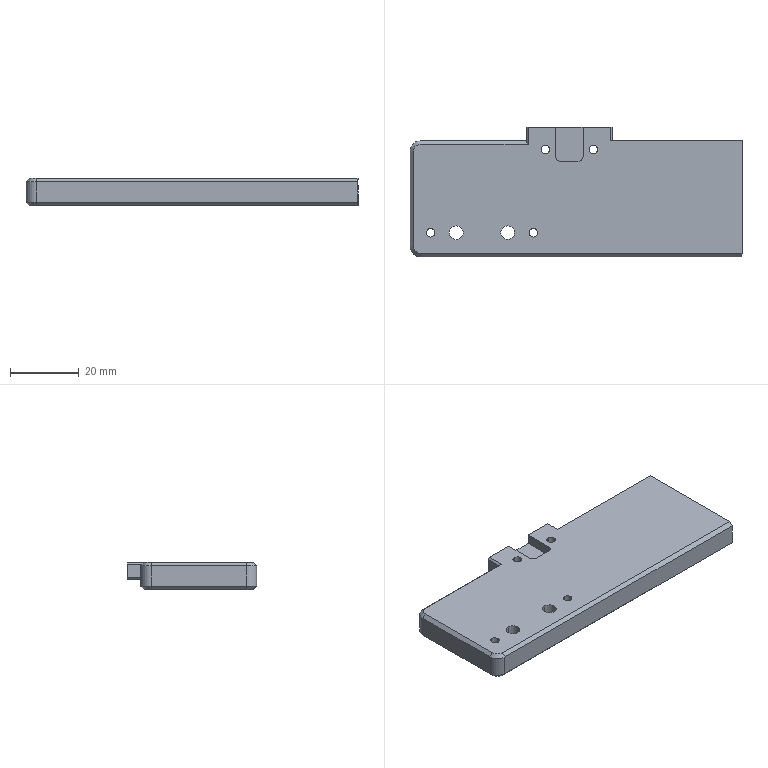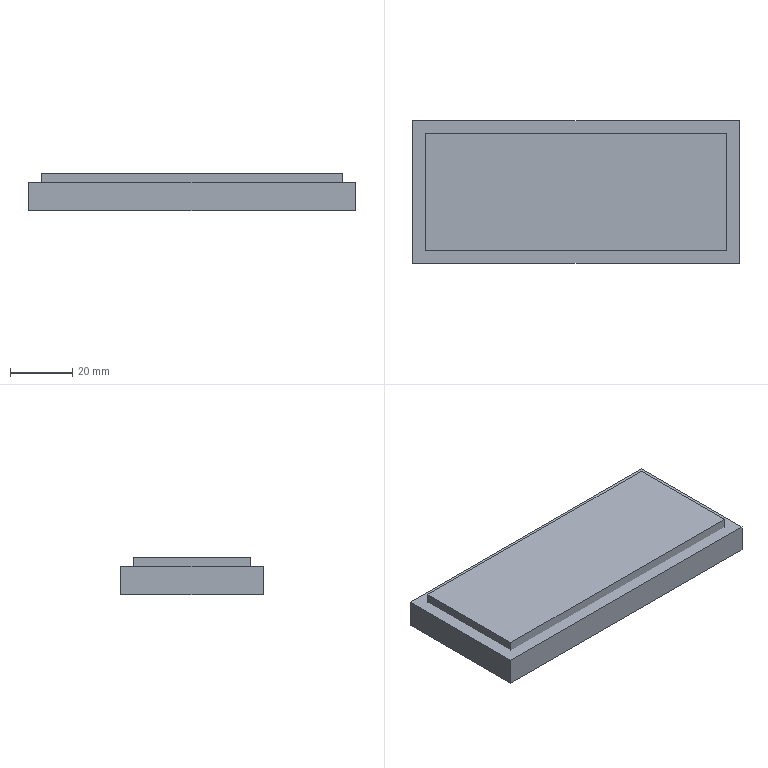CAM job | NX | 3+2 milling, drilling | part box 96.9 x 37.8 x 8 mm | stock box 104.9 x 45.8 x 12 mm
Tools:
number,name,description,diameter,corner_radius,flute_length,length,flutes
1,D50,Milling Tool-5 Parameters,50.0,0.0,50.0,75.0,2
7,D6A45,Milling Tool-5 Parameters,6.0,0.0,3.0,3.0,2
11,2.5ZT,Drilling Tool,2.5,0.0,35.0,50.0,2
14,4.0ZT,Drilling Tool,4.0,0.0,35.0,50.0,2
10,D10,Milling Tool-5 Parameters,10.0,0.0,50.0,75.0,2
6,D6,Milling Tool-5 Parameters,6.0,0.0,50.0,75.0,2
4,D4,Milling Tool-5 Parameters,4.0,0.0,50.0,75.0,2
5,D2,Milling Tool-5 Parameters,2.0,0.0,50.0,75.0,2
3,D3,Milling Tool-5 Parameters,3.0,0.0,50.0,75.0,2
13,3.4ZT,Drilling Tool,3.3,0.0,35.0,50.0,2
Operations:
program,operation,operation_type,tool,method,geometry_group,spindle_rpm,surface_speed,feed_per_tooth,feed_cut,feed_plunge,cut_length_mm,path_length_mm,cut_time_min,machine_time_min
1-12-40-100毛胚-虎钳,FLOOR_WALL,VolumeBased25DMillingOperation,D50,METHOD,A,6500.0,1286.0,0.0962,1250.0,100.0,166.9,220.9,0.1335,0.1389
1-12-40-100毛胚-虎钳,DRILLING_COPY_1,Operation,D6A45,METHOD,A,3000.0,56.0,0.0333,200.0,0.0,26.4,198.304,0.132,0.1492
1-12-40-100毛胚-虎钳,DRILLING_COPY_1_COPY_COPY_COPY_COPY_COPY,Operation,2.5ZT,METHOD,A,2000.0,15.0,0.0375,150.0,0.0,51.004,240.209,0.34,0.3589
1-12-40-100毛胚-虎钳,DRILLING_COPY_1_COPY_COPY_COPY_COPY_COPY_COPY,Operation,4.0ZT,METHOD,A,2000.0,15.0,0.0375,150.0,0.0,26.403,131.104,0.176,0.1865
1-12-40-100毛胚-虎钳,ADAPTIVE_MILLING,CavityMilling,D10,METHOD,A,7000.0,219.0,0.2143,3000.0,1000.0,2471.054,2677.109,0.8277,0.8483
1-12-40-100毛胚-虎钳,ZLEVEL_PROFILE_COPY_1,ZLevelMilling,D6,METHOD,A,7000.0,87.0,0.1071,1500.0,1000.0,491.126,870.557,0.3539,0.3919
1-12-40-100毛胚-虎钳,ZLEVEL_PROFILE_COPY_COPY_1_COPY_COPY_COPY_1,ZLevelMilling,D6,METHOD,A,7000.0,219.0,0.0714,1000.0,100.0,284.979,360.979,0.285,0.2926
1-12-40-100毛胚-虎钳,ZLEVEL_PROFILE_COPY_1_1,ZLevelMilling,D4,METHOD,A,7000.0,87.0,0.1071,1500.0,1000.0,260.364,704.653,0.1936,0.238
1-12-40-100毛胚-虎钳,ZLEVEL_PROFILE_COPY_1_COPY_COPY_COPY_COPY_2_COPY_COPY_1,ZLevelMilling,D6A45,METHOD,A,7000.0,131.0,0.0714,1000.0,1000.0,303.879,574.174,0.3039,0.3309
2-12-40-100毛胚-虎钳,FLOOR_WALL_COPY,VolumeBased25DMillingOperation,D50,METHOD,B,6500.0,1286.0,0.0962,1250.0,100.0,635.6,1298.301,0.5085,0.5748
2-12-40-100毛胚-虎钳,FLOOR_WALL_1,VolumeBased25DMillingOperation,D6,METHOD,B,7000.0,131.0,0.1429,2000.0,100.0,525.195,600.328,0.2626,0.2701
2-12-40-100毛胚-虎钳,HOLE_MILLING_COPY,CylinderMilling,D3,METHOD,B,7000.0,43.0,0.0786,1100.0,100.0,346.388,490.388,0.3149,0.3293
2-12-40-100毛胚-虎钳,ZLEVEL_PROFILE_COPY_1_COPY_COPY_COPY_COPY_2_COPY_COPY_1_1,ZLevelMilling,D6A45,METHOD,B,7000.0,131.0,0.0714,1000.0,1000.0,283.407,512.039,0.2834,0.3063
2-12-40-100毛胚-虎钳,ZLEVEL_PROFILE_COPY_1_COPY_COPY_COPY_COPY_2_COPY_COPY_1_1_COPY,ZLevelMilling,D6A45,METHOD,B,7000.0,131.0,0.0714,1000.0,1000.0,31.702,99.702,0.0317,0.0385
2-12-40-100毛胚-虎钳,DRILLING_COPY_1_COPY,Operation,D6A45,METHOD,B,3000.0,56.0,0.0333,200.0,0.0,17.6,173.401,0.088,0.1036
2-12-40-100毛胚-虎钳,刀补5,CylinderMilling,D3,METHOD,B,7000.0,43.0,0.0607,850.0,100.0,85.393,229.393,0.1005,0.1149
3-12-40-100毛胚-虎钳,DRILLING_COPY_1_COPY_1,Operation,D6A45,METHOD,C,3000.0,56.0,0.0333,200.0,0.0,23.75,146.162,0.1187,0.131
3-12-40-100毛胚-虎钳,DRILLING_COPY_1_COPY_COPY_COPY_COPY,Operation,3.4ZT,METHOD,C,2000.0,21.0,0.0375,150.0,0.0,70.467,239.596,0.4698,0.4867
3-12-40-100毛胚-虎钳,ZLEVEL_PROFILE,ZLevelMilling,D2,METHOD,C,7000.0,65.0,0.0786,1100.0,1000.0,985.461,1133.85,0.8999,0.9147
3-12-40-100毛胚-虎钳,ZLEVEL_PROFILE_COPY_1_COPY_COPY_COPY_COPY_2_COPY_COPY_1_1_COPY_1,ZLevelMilling,D6A45,METHOD,C,7000.0,131.0,0.0714,1000.0,1000.0,36.261,382.622,0.0363,0.0709
3-12-40-100毛胚-虎钳,刀补5.,ZLevelMilling,D2,METHOD,C,7000.0,65.0,0.0786,1100.0,1000.0,154.819,305.884,0.1409,0.156